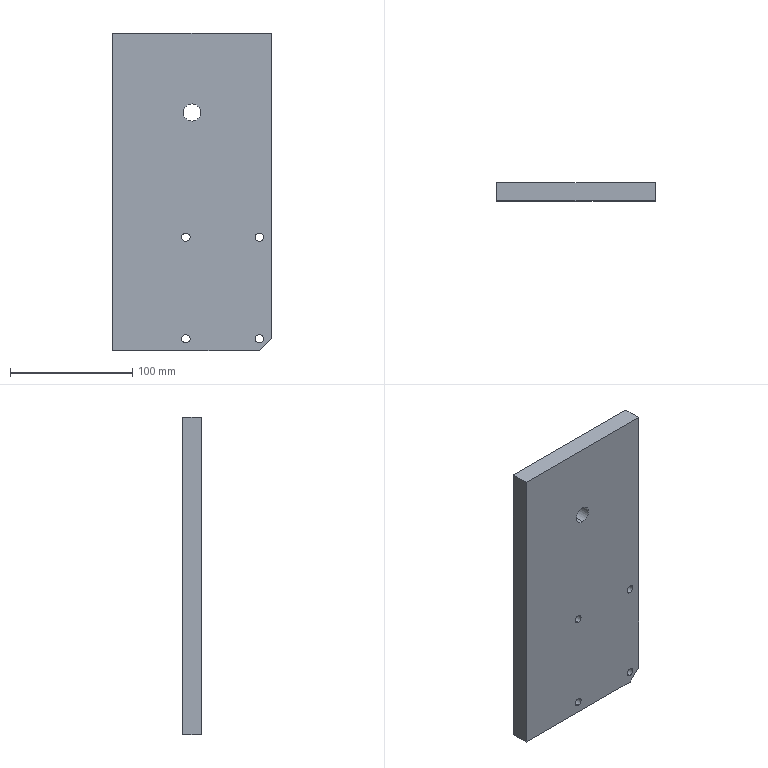Part | STEP file | PN_0001_default<by machining> | 1 solid | 17 faces | box 130 x 15 x 260 mm | volume 501762 mm3 | cylinder 10 | plane 7 | commonest cylinder face diameters 6.8 x8 14 x2
STEP:
#1=CARTESIAN_POINT('',(0.,0.,0.));
#2=DIRECTION('',(0.,0.,1.));
#3=DIRECTION('',(1.,0.,0.));
#4=AXIS2_PLACEMENT_3D('',#1,#2,#3);
#5=CARTESIAN_POINT('',(-180.,-25.,846.6));
#6=VERTEX_POINT('',#5);
#7=CARTESIAN_POINT('',(-180.,-40.,846.6));
#8=VERTEX_POINT('',#7);
#9=CARTESIAN_POINT('',(-180.,-40.,846.6));
#10=DIRECTION('',(0.,-1.,0.));
#11=VECTOR('',#10,1.);
#12=LINE('',#9,#11);
#13=CARTESIAN_POINT('',(-180.,-40.,850.));
#14=DIRECTION('',(0.,-1.,0.));
#15=DIRECTION('',(0.,0.,-1.));
#16=AXIS2_PLACEMENT_3D('',#13,#14,#15);
#17=CYLINDRICAL_SURFACE('',#16,3.4);
#18=CARTESIAN_POINT('',(6.283,0.));
#19=DIRECTION('',(0.,1.));
#20=VECTOR('',#19,1.);
#21=LINE('',#18,#20);
#22=(GEOMETRIC_REPRESENTATION_CONTEXT(2)PARAMETRIC_REPRESENTATION_CONTEXT()REPRESENTATION_CONTEXT('',''));
#23=DEFINITIONAL_REPRESENTATION('',(#21),#22);
#24=PCURVE('',#17,#23);
#25=CARTESIAN_POINT('',(-180.,-40.,850.));
#26=DIRECTION('',(0.,-1.,0.));
#27=DIRECTION('',(0.,0.,-1.));
#28=AXIS2_PLACEMENT_3D('',#25,#26,#27);
#29=CYLINDRICAL_SURFACE('',#28,3.4);
#30=CARTESIAN_POINT('',(0.,0.));
#31=DIRECTION('',(0.,1.));
#32=VECTOR('',#31,1.);
#33=LINE('',#30,#32);
#34=(GEOMETRIC_REPRESENTATION_CONTEXT(2)PARAMETRIC_REPRESENTATION_CONTEXT()REPRESENTATION_CONTEXT('',''));
#35=DEFINITIONAL_REPRESENTATION('',(#33),#34);
#36=PCURVE('',#29,#35);
#37=SURFACE_CURVE('',#12,(#24,#36),.PCURVE_S1.);
#38=EDGE_CURVE('',#6,#8,#37,.T.);
#39=ORIENTED_EDGE('',*,*,#38,.T.);
#40=CARTESIAN_POINT('',(-180.,-40.,853.4));
#41=VERTEX_POINT('',#40);
#42=CARTESIAN_POINT('',(-180.,-40.,850.));
#43=DIRECTION('',(0.,-1.,0.));
#44=DIRECTION('',(0.,0.,-1.));
#45=AXIS2_PLACEMENT_3D('',#42,#43,#44);
#46=CIRCLE('',#45,3.4);
#47=CARTESIAN_POINT('',(0.,0.));
#48=DIRECTION('',(1.,0.));
#49=VECTOR('',#48,1.);
#50=LINE('',#47,#49);
#51=(GEOMETRIC_REPRESENTATION_CONTEXT(2)PARAMETRIC_REPRESENTATION_CONTEXT()REPRESENTATION_CONTEXT('',''));
#52=DEFINITIONAL_REPRESENTATION('',(#50),#51);
#53=PCURVE('',#17,#52);
#54=CARTESIAN_POINT('',(0.,-40.,0.));
#55=DIRECTION('',(0.,-1.,0.));
#56=DIRECTION('',(0.,0.,-1.));
#57=AXIS2_PLACEMENT_3D('',#54,#55,#56);
#58=PLANE('',#57);
#59=CARTESIAN_POINT('',(-850.,-180.));
#60=DIRECTION('',(1.,0.));
#61=AXIS2_PLACEMENT_2D('',#59,#60);
#62=CIRCLE('',#61,3.4);
#63=(GEOMETRIC_REPRESENTATION_CONTEXT(2)PARAMETRIC_REPRESENTATION_CONTEXT()REPRESENTATION_CONTEXT('',''));
#64=DEFINITIONAL_REPRESENTATION('',(#62),#63);
#65=PCURVE('',#58,#64);
#66=SURFACE_CURVE('',#46,(#53,#65),.PCURVE_S1.);
#67=EDGE_CURVE('',#41,#8,#66,.T.);
#68=ORIENTED_EDGE('',*,*,#67,.F.);
#69=CARTESIAN_POINT('',(-180.,-25.,853.4));
#70=VERTEX_POINT('',#69);
#71=CARTESIAN_POINT('',(-180.,-40.,853.4));
#72=DIRECTION('',(0.,-1.,0.));
#73=VECTOR('',#72,1.);
#74=LINE('',#71,#73);
#75=CARTESIAN_POINT('',(3.142,0.));
#76=DIRECTION('',(0.,1.));
#77=VECTOR('',#76,1.);
#78=LINE('',#75,#77);
#79=(GEOMETRIC_REPRESENTATION_CONTEXT(2)PARAMETRIC_REPRESENTATION_CONTEXT()REPRESENTATION_CONTEXT('',''));
#80=DEFINITIONAL_REPRESENTATION('',(#78),#79);
#81=PCURVE('',#17,#80);
#82=CARTESIAN_POINT('',(3.142,0.));
#83=DIRECTION('',(0.,1.));
#84=VECTOR('',#83,1.);
#85=LINE('',#82,#84);
#86=(GEOMETRIC_REPRESENTATION_CONTEXT(2)PARAMETRIC_REPRESENTATION_CONTEXT()REPRESENTATION_CONTEXT('',''));
#87=DEFINITIONAL_REPRESENTATION('',(#85),#86);
#88=PCURVE('',#29,#87);
#89=SURFACE_CURVE('',#74,(#81,#88),.PCURVE_S1.);
#90=EDGE_CURVE('',#70,#41,#89,.T.);
#91=ORIENTED_EDGE('',*,*,#90,.F.);
#92=CARTESIAN_POINT('',(-180.,-25.,850.));
#93=DIRECTION('',(0.,-1.,0.));
#94=DIRECTION('',(0.,0.,-1.));
#95=AXIS2_PLACEMENT_3D('',#92,#93,#94);
#96=CIRCLE('',#95,3.4);
#97=CARTESIAN_POINT('',(0.,-15.));
#98=DIRECTION('',(1.,0.));
#99=VECTOR('',#98,1.);
#100=LINE('',#97,#99);
#101=(GEOMETRIC_REPRESENTATION_CONTEXT(2)PARAMETRIC_REPRESENTATION_CONTEXT()REPRESENTATION_CONTEXT('',''));
#102=DEFINITIONAL_REPRESENTATION('',(#100),#101);
#103=PCURVE('',#17,#102);
#104=CARTESIAN_POINT('',(0.,-25.,0.));
#105=DIRECTION('',(0.,-1.,0.));
#106=DIRECTION('',(0.,0.,-1.));
#107=AXIS2_PLACEMENT_3D('',#104,#105,#106);
#108=PLANE('',#107);
#109=CARTESIAN_POINT('',(-850.,-180.));
#110=DIRECTION('',(1.,0.));
#111=AXIS2_PLACEMENT_2D('',#109,#110);
#112=CIRCLE('',#111,3.4);
#113=(GEOMETRIC_REPRESENTATION_CONTEXT(2)PARAMETRIC_REPRESENTATION_CONTEXT()REPRESENTATION_CONTEXT('',''));
#114=DEFINITIONAL_REPRESENTATION('',(#112),#113);
#115=PCURVE('',#108,#114);
#116=SURFACE_CURVE('',#96,(#103,#115),.PCURVE_S1.);
#117=EDGE_CURVE('',#70,#6,#116,.T.);
#118=ORIENTED_EDGE('',*,*,#117,.T.);
#119=EDGE_LOOP('',(#39,#68,#91,#118));
#120=FACE_BOUND('',#119,.F.);
#121=ADVANCED_FACE('',(#120),#17,.F.);
#122=CARTESIAN_POINT('',(-180.,-25.,929.6));
#123=VERTEX_POINT('',#122);
#124=CARTESIAN_POINT('',(-180.,-40.,929.6));
#125=VERTEX_POINT('',#124);
#126=CARTESIAN_POINT('',(-180.,-40.,929.6));
#127=DIRECTION('',(0.,-1.,0.));
#128=VECTOR('',#127,1.);
#129=LINE('',#126,#128);
#130=CARTESIAN_POINT('',(-180.,-40.,933.));
#131=DIRECTION('',(0.,-1.,0.));
#132=DIRECTION('',(0.,0.,-1.));
#133=AXIS2_PLACEMENT_3D('',#130,#131,#132);
#134=CYLINDRICAL_SURFACE('',#133,3.4);
#135=CARTESIAN_POINT('',(6.283,0.));
#136=DIRECTION('',(0.,1.));
#137=VECTOR('',#136,1.);
#138=LINE('',#135,#137);
#139=(GEOMETRIC_REPRESENTATION_CONTEXT(2)PARAMETRIC_REPRESENTATION_CONTEXT()REPRESENTATION_CONTEXT('',''));
#140=DEFINITIONAL_REPRESENTATION('',(#138),#139);
#141=PCURVE('',#134,#140);
#142=CARTESIAN_POINT('',(-180.,-40.,933.));
#143=DIRECTION('',(0.,-1.,0.));
#144=DIRECTION('',(0.,0.,-1.));
#145=AXIS2_PLACEMENT_3D('',#142,#143,#144);
#146=CYLINDRICAL_SURFACE('',#145,3.4);
#147=CARTESIAN_POINT('',(0.,0.));
#148=DIRECTION('',(0.,1.));
#149=VECTOR('',#148,1.);
#150=LINE('',#147,#149);
#151=(GEOMETRIC_REPRESENTATION_CONTEXT(2)PARAMETRIC_REPRESENTATION_CONTEXT()REPRESENTATION_CONTEXT('',''));
#152=DEFINITIONAL_REPRESENTATION('',(#150),#151);
#153=PCURVE('',#146,#152);
#154=SURFACE_CURVE('',#129,(#141,#153),.PCURVE_S1.);
#155=EDGE_CURVE('',#123,#125,#154,.T.);
#156=ORIENTED_EDGE('',*,*,#155,.T.);
#157=CARTESIAN_POINT('',(-180.,-40.,936.4));
#158=VERTEX_POINT('',#157);
#159=CARTESIAN_POINT('',(-180.,-40.,933.));
#160=DIRECTION('',(0.,-1.,0.));
#161=DIRECTION('',(0.,0.,-1.));
#162=AXIS2_PLACEMENT_3D('',#159,#160,#161);
#163=CIRCLE('',#162,3.4);
#164=CARTESIAN_POINT('',(0.,0.));
#165=DIRECTION('',(1.,0.));
#166=VECTOR('',#165,1.);
#167=LINE('',#164,#166);
#168=(GEOMETRIC_REPRESENTATION_CONTEXT(2)PARAMETRIC_REPRESENTATION_CONTEXT()REPRESENTATION_CONTEXT('',''));
#169=DEFINITIONAL_REPRESENTATION('',(#167),#168);
#170=PCURVE('',#134,#169);
#171=CARTESIAN_POINT('',(-933.,-180.));
#172=DIRECTION('',(1.,0.));
#173=AXIS2_PLACEMENT_2D('',#171,#172);
#174=CIRCLE('',#173,3.4);
#175=(GEOMETRIC_REPRESENTATION_CONTEXT(2)PARAMETRIC_REPRESENTATION_CONTEXT()REPRESENTATION_CONTEXT('',''));
#176=DEFINITIONAL_REPRESENTATION('',(#174),#175);
#177=PCURVE('',#58,#176);
#178=SURFACE_CURVE('',#163,(#170,#177),.PCURVE_S1.);
#179=EDGE_CURVE('',#158,#125,#178,.T.);
#180=ORIENTED_EDGE('',*,*,#179,.F.);
#181=CARTESIAN_POINT('',(-180.,-25.,936.4));
#182=VERTEX_POINT('',#181);
#183=CARTESIAN_POINT('',(-180.,-40.,936.4));
#184=DIRECTION('',(0.,-1.,0.));
#185=VECTOR('',#184,1.);
#186=LINE('',#183,#185);
#187=CARTESIAN_POINT('',(3.142,0.));
#188=DIRECTION('',(0.,1.));
#189=VECTOR('',#188,1.);
#190=LINE('',#187,#189);
#191=(GEOMETRIC_REPRESENTATION_CONTEXT(2)PARAMETRIC_REPRESENTATION_CONTEXT()REPRESENTATION_CONTEXT('',''));
#192=DEFINITIONAL_REPRESENTATION('',(#190),#191);
#193=PCURVE('',#134,#192);
#194=CARTESIAN_POINT('',(3.142,0.));
#195=DIRECTION('',(0.,1.));
#196=VECTOR('',#195,1.);
#197=LINE('',#194,#196);
#198=(GEOMETRIC_REPRESENTATION_CONTEXT(2)PARAMETRIC_REPRESENTATION_CONTEXT()REPRESENTATION_CONTEXT('',''));
#199=DEFINITIONAL_REPRESENTATION('',(#197),#198);
#200=PCURVE('',#146,#199);
#201=SURFACE_CURVE('',#186,(#193,#200),.PCURVE_S1.);
#202=EDGE_CURVE('',#182,#158,#201,.T.);
#203=ORIENTED_EDGE('',*,*,#202,.F.);
#204=CARTESIAN_POINT('',(-180.,-25.,933.));
#205=DIRECTION('',(0.,-1.,0.));
#206=DIRECTION('',(0.,0.,-1.));
#207=AXIS2_PLACEMENT_3D('',#204,#205,#206);
#208=CIRCLE('',#207,3.4);
#209=CARTESIAN_POINT('',(0.,-15.));
#210=DIRECTION('',(1.,0.));
#211=VECTOR('',#210,1.);
#212=LINE('',#209,#211);
#213=(GEOMETRIC_REPRESENTATION_CONTEXT(2)PARAMETRIC_REPRESENTATION_CONTEXT()REPRESENTATION_CONTEXT('',''));
#214=DEFINITIONAL_REPRESENTATION('',(#212),#213);
#215=PCURVE('',#134,#214);
#216=CARTESIAN_POINT('',(-933.,-180.));
#217=DIRECTION('',(1.,0.));
#218=AXIS2_PLACEMENT_2D('',#216,#217);
#219=CIRCLE('',#218,3.4);
#220=(GEOMETRIC_REPRESENTATION_CONTEXT(2)PARAMETRIC_REPRESENTATION_CONTEXT()REPRESENTATION_CONTEXT('',''));
#221=DEFINITIONAL_REPRESENTATION('',(#219),#220);
#222=PCURVE('',#108,#221);
#223=SURFACE_CURVE('',#208,(#215,#222),.PCURVE_S1.);
#224=EDGE_CURVE('',#182,#123,#223,.T.);
#225=ORIENTED_EDGE('',*,*,#224,.T.);
#226=EDGE_LOOP('',(#156,#180,#203,#225));
#227=FACE_BOUND('',#226,.F.);
#228=ADVANCED_FACE('',(#227),#134,.F.);
#229=CARTESIAN_POINT('',(-240.,-25.,929.6));
#230=VERTEX_POINT('',#229);
#231=CARTESIAN_POINT('',(-240.,-40.,929.6));
#232=VERTEX_POINT('',#231);
#233=CARTESIAN_POINT('',(-240.,-40.,929.6));
#234=DIRECTION('',(0.,-1.,0.));
#235=VECTOR('',#234,1.);
#236=LINE('',#233,#235);
#237=CARTESIAN_POINT('',(-240.,-40.,933.));
#238=DIRECTION('',(0.,-1.,0.));
#239=DIRECTION('',(0.,0.,-1.));
#240=AXIS2_PLACEMENT_3D('',#237,#238,#239);
#241=CYLINDRICAL_SURFACE('',#240,3.4);
#242=CARTESIAN_POINT('',(6.283,0.));
#243=DIRECTION('',(0.,1.));
#244=VECTOR('',#243,1.);
#245=LINE('',#242,#244);
#246=(GEOMETRIC_REPRESENTATION_CONTEXT(2)PARAMETRIC_REPRESENTATION_CONTEXT()REPRESENTATION_CONTEXT('',''));
#247=DEFINITIONAL_REPRESENTATION('',(#245),#246);
#248=PCURVE('',#241,#247);
#249=CARTESIAN_POINT('',(-240.,-40.,933.));
#250=DIRECTION('',(0.,-1.,0.));
#251=DIRECTION('',(0.,0.,-1.));
#252=AXIS2_PLACEMENT_3D('',#249,#250,#251);
#253=CYLINDRICAL_SURFACE('',#252,3.4);
#254=CARTESIAN_POINT('',(0.,0.));
#255=DIRECTION('',(0.,1.));
#256=VECTOR('',#255,1.);
#257=LINE('',#254,#256);
#258=(GEOMETRIC_REPRESENTATION_CONTEXT(2)PARAMETRIC_REPRESENTATION_CONTEXT()REPRESENTATION_CONTEXT('',''));
#259=DEFINITIONAL_REPRESENTATION('',(#257),#258);
#260=PCURVE('',#253,#259);
#261=SURFACE_CURVE('',#236,(#248,#260),.PCURVE_S1.);
#262=EDGE_CURVE('',#230,#232,#261,.T.);
#263=ORIENTED_EDGE('',*,*,#262,.T.);
#264=CARTESIAN_POINT('',(-240.,-40.,936.4));
#265=VERTEX_POINT('',#264);
#266=CARTESIAN_POINT('',(-240.,-40.,933.));
#267=DIRECTION('',(0.,-1.,0.));
#268=DIRECTION('',(0.,0.,-1.));
#269=AXIS2_PLACEMENT_3D('',#266,#267,#268);
#270=CIRCLE('',#269,3.4);
#271=CARTESIAN_POINT('',(0.,0.));
#272=DIRECTION('',(1.,0.));
#273=VECTOR('',#272,1.);
#274=LINE('',#271,#273);
#275=(GEOMETRIC_REPRESENTATION_CONTEXT(2)PARAMETRIC_REPRESENTATION_CONTEXT()REPRESENTATION_CONTEXT('',''));
#276=DEFINITIONAL_REPRESENTATION('',(#274),#275);
#277=PCURVE('',#241,#276);
#278=CARTESIAN_POINT('',(-933.,-240.));
#279=DIRECTION('',(1.,0.));
#280=AXIS2_PLACEMENT_2D('',#278,#279);
#281=CIRCLE('',#280,3.4);
#282=(GEOMETRIC_REPRESENTATION_CONTEXT(2)PARAMETRIC_REPRESENTATION_CONTEXT()REPRESENTATION_CONTEXT('',''));
#283=DEFINITIONAL_REPRESENTATION('',(#281),#282);
#284=PCURVE('',#58,#283);
#285=SURFACE_CURVE('',#270,(#277,#284),.PCURVE_S1.);
#286=EDGE_CURVE('',#265,#232,#285,.T.);
#287=ORIENTED_EDGE('',*,*,#286,.F.);
#288=CARTESIAN_POINT('',(-240.,-25.,936.4));
#289=VERTEX_POINT('',#288);
#290=CARTESIAN_POINT('',(-240.,-40.,936.4));
#291=DIRECTION('',(0.,-1.,0.));
#292=VECTOR('',#291,1.);
#293=LINE('',#290,#292);
#294=CARTESIAN_POINT('',(3.142,0.));
#295=DIRECTION('',(0.,1.));
#296=VECTOR('',#295,1.);
#297=LINE('',#294,#296);
#298=(GEOMETRIC_REPRESENTATION_CONTEXT(2)PARAMETRIC_REPRESENTATION_CONTEXT()REPRESENTATION_CONTEXT('',''));
#299=DEFINITIONAL_REPRESENTATION('',(#297),#298);
#300=PCURVE('',#241,#299);
#301=CARTESIAN_POINT('',(3.142,0.));
#302=DIRECTION('',(0.,1.));
#303=VECTOR('',#302,1.);
#304=LINE('',#301,#303);
#305=(GEOMETRIC_REPRESENTATION_CONTEXT(2)PARAMETRIC_REPRESENTATION_CONTEXT()REPRESENTATION_CONTEXT('',''));
#306=DEFINITIONAL_REPRESENTATION('',(#304),#305);
#307=PCURVE('',#253,#306);
#308=SURFACE_CURVE('',#293,(#300,#307),.PCURVE_S1.);
#309=EDGE_CURVE('',#289,#265,#308,.T.);
#310=ORIENTED_EDGE('',*,*,#309,.F.);
#311=CARTESIAN_POINT('',(-240.,-25.,933.));
#312=DIRECTION('',(0.,-1.,0.));
#313=DIRECTION('',(0.,0.,-1.));
#314=AXIS2_PLACEMENT_3D('',#311,#312,#313);
#315=CIRCLE('',#314,3.4);
#316=CARTESIAN_POINT('',(0.,-15.));
#317=DIRECTION('',(1.,0.));
#318=VECTOR('',#317,1.);
#319=LINE('',#316,#318);
#320=(GEOMETRIC_REPRESENTATION_CONTEXT(2)PARAMETRIC_REPRESENTATION_CONTEXT()REPRESENTATION_CONTEXT('',''));
#321=DEFINITIONAL_REPRESENTATION('',(#319),#320);
#322=PCURVE('',#241,#321);
#323=CARTESIAN_POINT('',(-933.,-240.));
#324=DIRECTION('',(1.,0.));
#325=AXIS2_PLACEMENT_2D('',#323,#324);
#326=CIRCLE('',#325,3.4);
#327=(GEOMETRIC_REPRESENTATION_CONTEXT(2)PARAMETRIC_REPRESENTATION_CONTEXT()REPRESENTATION_CONTEXT('',''));
#328=DEFINITIONAL_REPRESENTATION('',(#326),#327);
#329=PCURVE('',#108,#328);
#330=SURFACE_CURVE('',#315,(#322,#329),.PCURVE_S1.);
#331=EDGE_CURVE('',#289,#230,#330,.T.);
#332=ORIENTED_EDGE('',*,*,#331,.T.);
#333=EDGE_LOOP('',(#263,#287,#310,#332));
#334=FACE_BOUND('',#333,.F.);
#335=ADVANCED_FACE('',(#334),#241,.F.);
#336=CARTESIAN_POINT('',(-240.,-25.,846.6));
#337=VERTEX_POINT('',#336);
#338=CARTESIAN_POINT('',(-240.,-40.,846.6));
#339=VERTEX_POINT('',#338);
#340=CARTESIAN_POINT('',(-240.,-40.,846.6));
#341=DIRECTION('',(0.,-1.,0.));
#342=VECTOR('',#341,1.);
#343=LINE('',#340,#342);
#344=CARTESIAN_POINT('',(-240.,-40.,850.));
#345=DIRECTION('',(0.,-1.,0.));
#346=DIRECTION('',(0.,0.,-1.));
#347=AXIS2_PLACEMENT_3D('',#344,#345,#346);
#348=CYLINDRICAL_SURFACE('',#347,3.4);
#349=CARTESIAN_POINT('',(6.283,0.));
#350=DIRECTION('',(0.,1.));
#351=VECTOR('',#350,1.);
#352=LINE('',#349,#351);
#353=(GEOMETRIC_REPRESENTATION_CONTEXT(2)PARAMETRIC_REPRESENTATION_CONTEXT()REPRESENTATION_CONTEXT('',''));
#354=DEFINITIONAL_REPRESENTATION('',(#352),#353);
#355=PCURVE('',#348,#354);
#356=CARTESIAN_POINT('',(-240.,-40.,850.));
#357=DIRECTION('',(0.,-1.,0.));
#358=DIRECTION('',(0.,0.,-1.));
#359=AXIS2_PLACEMENT_3D('',#356,#357,#358);
#360=CYLINDRICAL_SURFACE('',#359,3.4);
#361=CARTESIAN_POINT('',(0.,0.));
#362=DIRECTION('',(0.,1.));
#363=VECTOR('',#362,1.);
#364=LINE('',#361,#363);
#365=(GEOMETRIC_REPRESENTATION_CONTEXT(2)PARAMETRIC_REPRESENTATION_CONTEXT()REPRESENTATION_CONTEXT('',''));
#366=DEFINITIONAL_REPRESENTATION('',(#364),#365);
#367=PCURVE('',#360,#366);
#368=SURFACE_CURVE('',#343,(#355,#367),.PCURVE_S1.);
#369=EDGE_CURVE('',#337,#339,#368,.T.);
#370=ORIENTED_EDGE('',*,*,#369,.T.);
#371=CARTESIAN_POINT('',(-240.,-40.,853.4));
#372=VERTEX_POINT('',#371);
#373=CARTESIAN_POINT('',(-240.,-40.,850.));
#374=DIRECTION('',(0.,-1.,0.));
#375=DIRECTION('',(0.,0.,-1.));
#376=AXIS2_PLACEMENT_3D('',#373,#374,#375);
#377=CIRCLE('',#376,3.4);
#378=CARTESIAN_POINT('',(0.,0.));
#379=DIRECTION('',(1.,0.));
#380=VECTOR('',#379,1.);
#381=LINE('',#378,#380);
#382=(GEOMETRIC_REPRESENTATION_CONTEXT(2)PARAMETRIC_REPRESENTATION_CONTEXT()REPRESENTATION_CONTEXT('',''));
#383=DEFINITIONAL_REPRESENTATION('',(#381),#382);
#384=PCURVE('',#348,#383);
#385=CARTESIAN_POINT('',(-850.,-240.));
#386=DIRECTION('',(1.,0.));
#387=AXIS2_PLACEMENT_2D('',#385,#386);
#388=CIRCLE('',#387,3.4);
#389=(GEOMETRIC_REPRESENTATION_CONTEXT(2)PARAMETRIC_REPRESENTATION_CONTEXT()REPRESENTATION_CONTEXT('',''));
#390=DEFINITIONAL_REPRESENTATION('',(#388),#389);
#391=PCURVE('',#58,#390);
#392=SURFACE_CURVE('',#377,(#384,#391),.PCURVE_S1.);
#393=EDGE_CURVE('',#372,#339,#392,.T.);
#394=ORIENTED_EDGE('',*,*,#393,.F.);
#395=CARTESIAN_POINT('',(-240.,-25.,853.4));
#396=VERTEX_POINT('',#395);
#397=CARTESIAN_POINT('',(-240.,-40.,853.4));
#398=DIRECTION('',(0.,-1.,0.));
#399=VECTOR('',#398,1.);
#400=LINE('',#397,#399);
#401=CARTESIAN_POINT('',(3.142,0.));
#402=DIRECTION('',(0.,1.));
#403=VECTOR('',#402,1.);
#404=LINE('',#401,#403);
#405=(GEOMETRIC_REPRESENTATION_CONTEXT(2)PARAMETRIC_REPRESENTATION_CONTEXT()REPRESENTATION_CONTEXT('',''));
#406=DEFINITIONAL_REPRESENTATION('',(#404),#405);
#407=PCURVE('',#348,#406);
#408=CARTESIAN_POINT('',(3.142,0.));
#409=DIRECTION('',(0.,1.));
#410=VECTOR('',#409,1.);
#411=LINE('',#408,#410);
#412=(GEOMETRIC_REPRESENTATION_CONTEXT(2)PARAMETRIC_REPRESENTATION_CONTEXT()REPRESENTATION_CONTEXT('',''));
#413=DEFINITIONAL_REPRESENTATION('',(#411),#412);
#414=PCURVE('',#360,#413);
#415=SURFACE_CURVE('',#400,(#407,#414),.PCURVE_S1.);
#416=EDGE_CURVE('',#396,#372,#415,.T.);
#417=ORIENTED_EDGE('',*,*,#416,.F.);
#418=CARTESIAN_POINT('',(-240.,-25.,850.));
#419=DIRECTION('',(0.,-1.,0.));
#420=DIRECTION('',(0.,0.,-1.));
#421=AXIS2_PLACEMENT_3D('',#418,#419,#420);
#422=CIRCLE('',#421,3.4);
#423=CARTESIAN_POINT('',(0.,-15.));
#424=DIRECTION('',(1.,0.));
#425=VECTOR('',#424,1.);
#426=LINE('',#423,#425);
#427=(GEOMETRIC_REPRESENTATION_CONTEXT(2)PARAMETRIC_REPRESENTATION_CONTEXT()REPRESENTATION_CONTEXT('',''));
#428=DEFINITIONAL_REPRESENTATION('',(#426),#427);
#429=PCURVE('',#348,#428);
#430=CARTESIAN_POINT('',(-850.,-240.));
#431=DIRECTION('',(1.,0.));
#432=AXIS2_PLACEMENT_2D('',#430,#431);
#433=CIRCLE('',#432,3.4);
#434=(GEOMETRIC_REPRESENTATION_CONTEXT(2)PARAMETRIC_REPRESENTATION_CONTEXT()REPRESENTATION_CONTEXT('',''));
#435=DEFINITIONAL_REPRESENTATION('',(#433),#434);
#436=PCURVE('',#108,#435);
#437=SURFACE_CURVE('',#422,(#429,#436),.PCURVE_S1.);
#438=EDGE_CURVE('',#396,#337,#437,.T.);
#439=ORIENTED_EDGE('',*,*,#438,.T.);
#440=EDGE_LOOP('',(#370,#394,#417,#439));
#441=FACE_BOUND('',#440,.F.);
#442=ADVANCED_FACE('',(#441),#348,.F.);
#443=CARTESIAN_POINT('',(-235.,-25.,1028.));
#444=VERTEX_POINT('',#443);
#445=CARTESIAN_POINT('',(-235.,-40.,1028.));
#446=VERTEX_POINT('',#445);
#447=CARTESIAN_POINT('',(-235.,-40.,1028.));
#448=DIRECTION('',(0.,-1.,0.));
#449=VECTOR('',#448,1.);
#450=LINE('',#447,#449);
#451=CARTESIAN_POINT('',(-235.,-40.,1035.));
#452=DIRECTION('',(0.,-1.,0.));
#453=DIRECTION('',(0.,0.,-1.));
#454=AXIS2_PLACEMENT_3D('',#451,#452,#453);
#455=CYLINDRICAL_SURFACE('',#454,7.);
#456=CARTESIAN_POINT('',(6.283,0.));
#457=DIRECTION('',(0.,1.));
#458=VECTOR('',#457,1.);
#459=LINE('',#456,#458);
#460=(GEOMETRIC_REPRESENTATION_CONTEXT(2)PARAMETRIC_REPRESENTATION_CONTEXT()REPRESENTATION_CONTEXT('',''));
#461=DEFINITIONAL_REPRESENTATION('',(#459),#460);
#462=PCURVE('',#455,#461);
#463=CARTESIAN_POINT('',(-235.,-40.,1035.));
#464=DIRECTION('',(0.,-1.,0.));
#465=DIRECTION('',(0.,0.,-1.));
#466=AXIS2_PLACEMENT_3D('',#463,#464,#465);
#467=CYLINDRICAL_SURFACE('',#466,7.);
#468=CARTESIAN_POINT('',(0.,0.));
#469=DIRECTION('',(0.,1.));
#470=VECTOR('',#469,1.);
#471=LINE('',#468,#470);
#472=(GEOMETRIC_REPRESENTATION_CONTEXT(2)PARAMETRIC_REPRESENTATION_CONTEXT()REPRESENTATION_CONTEXT('',''));
#473=DEFINITIONAL_REPRESENTATION('',(#471),#472);
#474=PCURVE('',#467,#473);
#475=SURFACE_CURVE('',#450,(#462,#474),.PCURVE_S1.);
#476=EDGE_CURVE('',#444,#446,#475,.T.);
#477=ORIENTED_EDGE('',*,*,#476,.T.);
#478=CARTESIAN_POINT('',(-235.,-40.,1042.));
#479=VERTEX_POINT('',#478);
#480=CARTESIAN_POINT('',(-235.,-40.,1035.));
#481=DIRECTION('',(0.,-1.,0.));
#482=DIRECTION('',(0.,0.,-1.));
#483=AXIS2_PLACEMENT_3D('',#480,#481,#482);
#484=CIRCLE('',#483,7.);
#485=CARTESIAN_POINT('',(0.,0.));
#486=DIRECTION('',(1.,0.));
#487=VECTOR('',#486,1.);
#488=LINE('',#485,#487);
#489=(GEOMETRIC_REPRESENTATION_CONTEXT(2)PARAMETRIC_REPRESENTATION_CONTEXT()REPRESENTATION_CONTEXT('',''));
#490=DEFINITIONAL_REPRESENTATION('',(#488),#489);
#491=PCURVE('',#455,#490);
#492=CARTESIAN_POINT('',(-1035.,-235.));
#493=DIRECTION('',(1.,0.));
#494=AXIS2_PLACEMENT_2D('',#492,#493);
#495=CIRCLE('',#494,7.);
#496=(GEOMETRIC_REPRESENTATION_CONTEXT(2)PARAMETRIC_REPRESENTATION_CONTEXT()REPRESENTATION_CONTEXT('',''));
#497=DEFINITIONAL_REPRESENTATION('',(#495),#496);
#498=PCURVE('',#58,#497);
#499=SURFACE_CURVE('',#484,(#491,#498),.PCURVE_S1.);
#500=EDGE_CURVE('',#479,#446,#499,.T.);
#501=ORIENTED_EDGE('',*,*,#500,.F.);
#502=CARTESIAN_POINT('',(-235.,-25.,1042.));
#503=VERTEX_POINT('',#502);
#504=CARTESIAN_POINT('',(-235.,-40.,1042.));
#505=DIRECTION('',(0.,-1.,0.));
#506=VECTOR('',#505,1.);
#507=LINE('',#504,#506);
#508=CARTESIAN_POINT('',(3.142,0.));
#509=DIRECTION('',(0.,1.));
#510=VECTOR('',#509,1.);
#511=LINE('',#508,#510);
#512=(GEOMETRIC_REPRESENTATION_CONTEXT(2)PARAMETRIC_REPRESENTATION_CONTEXT()REPRESENTATION_CONTEXT('',''));
#513=DEFINITIONAL_REPRESENTATION('',(#511),#512);
#514=PCURVE('',#455,#513);
#515=CARTESIAN_POINT('',(3.142,0.));
#516=DIRECTION('',(0.,1.));
#517=VECTOR('',#516,1.);
#518=LINE('',#515,#517);
#519=(GEOMETRIC_REPRESENTATION_CONTEXT(2)PARAMETRIC_REPRESENTATION_CONTEXT()REPRESENTATION_CONTEXT('',''));
#520=DEFINITIONAL_REPRESENTATION('',(#518),#519);
#521=PCURVE('',#467,#520);
#522=SURFACE_CURVE('',#507,(#514,#521),.PCURVE_S1.);
#523=EDGE_CURVE('',#503,#479,#522,.T.);
#524=ORIENTED_EDGE('',*,*,#523,.F.);
#525=CARTESIAN_POINT('',(-235.,-25.,1035.));
#526=DIRECTION('',(0.,-1.,0.));
#527=DIRECTION('',(0.,0.,-1.));
#528=AXIS2_PLACEMENT_3D('',#525,#526,#527);
#529=CIRCLE('',#528,7.);
#530=CARTESIAN_POINT('',(0.,-15.));
#531=DIRECTION('',(1.,0.));
#532=VECTOR('',#531,1.);
#533=LINE('',#530,#532);
#534=(GEOMETRIC_REPRESENTATION_CONTEXT(2)PARAMETRIC_REPRESENTATION_CONTEXT()REPRESENTATION_CONTEXT('',''));
#535=DEFINITIONAL_REPRESENTATION('',(#533),#534);
#536=PCURVE('',#455,#535);
#537=CARTESIAN_POINT('',(-1035.,-235.));
#538=DIRECTION('',(1.,0.));
#539=AXIS2_PLACEMENT_2D('',#537,#538);
#540=CIRCLE('',#539,7.);
#541=(GEOMETRIC_REPRESENTATION_CONTEXT(2)PARAMETRIC_REPRESENTATION_CONTEXT()REPRESENTATION_CONTEXT('',''));
#542=DEFINITIONAL_REPRESENTATION('',(#540),#541);
#543=PCURVE('',#108,#542);
#544=SURFACE_CURVE('',#529,(#536,#543),.PCURVE_S1.);
#545=EDGE_CURVE('',#503,#444,#544,.T.);
#546=ORIENTED_EDGE('',*,*,#545,.T.);
#547=EDGE_LOOP('',(#477,#501,#524,#546));
#548=FACE_BOUND('',#547,.F.);
#549=ADVANCED_FACE('',(#548),#455,.F.);
#550=CARTESIAN_POINT('',(-300.,-25.,1100.));
#551=VERTEX_POINT('',#550);
#552=CARTESIAN_POINT('',(-300.,-25.,840.));
#553=VERTEX_POINT('',#552);
#554=CARTESIAN_POINT('',(-300.,-25.,1100.));
#555=DIRECTION('',(0.,0.,-1.));
#556=VECTOR('',#555,1.);
#557=LINE('',#554,#556);
#558=CARTESIAN_POINT('',(-300.,-40.,1100.));
#559=DIRECTION('',(1.,0.,0.));
#560=DIRECTION('',(0.,1.,0.));
#561=AXIS2_PLACEMENT_3D('',#558,#559,#560);
#562=PLANE('',#561);
#563=CARTESIAN_POINT('',(15.,0.));
#564=DIRECTION('',(0.,-1.));
#565=VECTOR('',#564,1.);
#566=LINE('',#563,#565);
#567=(GEOMETRIC_REPRESENTATION_CONTEXT(2)PARAMETRIC_REPRESENTATION_CONTEXT()REPRESENTATION_CONTEXT('',''));
#568=DEFINITIONAL_REPRESENTATION('',(#566),#567);
#569=PCURVE('',#562,#568);
#570=CARTESIAN_POINT('',(-1100.,-300.));
#571=DIRECTION('',(1.,0.));
#572=VECTOR('',#571,1.);
#573=LINE('',#570,#572);
#574=(GEOMETRIC_REPRESENTATION_CONTEXT(2)PARAMETRIC_REPRESENTATION_CONTEXT()REPRESENTATION_CONTEXT('',''));
#575=DEFINITIONAL_REPRESENTATION('',(#573),#574);
#576=PCURVE('',#108,#575);
#577=SURFACE_CURVE('',#557,(#569,#576),.PCURVE_S1.);
#578=EDGE_CURVE('',#551,#553,#577,.T.);
#579=ORIENTED_EDGE('',*,*,#578,.T.);
#580=CARTESIAN_POINT('',(-300.,-40.,840.));
#581=VERTEX_POINT('',#580);
#582=CARTESIAN_POINT('',(-300.,-40.,840.));
#583=DIRECTION('',(0.,1.,0.));
#584=VECTOR('',#583,1.);
#585=LINE('',#582,#584);
#586=CARTESIAN_POINT('',(0.,-260.));
#587=DIRECTION('',(1.,0.));
#588=VECTOR('',#587,1.);
#589=LINE('',#586,#588);
#590=(GEOMETRIC_REPRESENTATION_CONTEXT(2)PARAMETRIC_REPRESENTATION_CONTEXT()REPRESENTATION_CONTEXT('',''));
#591=DEFINITIONAL_REPRESENTATION('',(#589),#590);
#592=PCURVE('',#562,#591);
#593=CARTESIAN_POINT('',(-300.,-40.,840.));
#594=DIRECTION('',(0.,0.,1.));
#595=DIRECTION('',(0.,-1.,0.));
#596=AXIS2_PLACEMENT_3D('',#593,#594,#595);
#597=PLANE('',#596);
#598=CARTESIAN_POINT('',(0.,0.));
#599=DIRECTION('',(-1.,0.));
#600=VECTOR('',#599,1.);
#601=LINE('',#598,#600);
#602=(GEOMETRIC_REPRESENTATION_CONTEXT(2)PARAMETRIC_REPRESENTATION_CONTEXT()REPRESENTATION_CONTEXT('',''));
#603=DEFINITIONAL_REPRESENTATION('',(#601),#602);
#604=PCURVE('',#597,#603);
#605=SURFACE_CURVE('',#585,(#592,#604),.PCURVE_S1.);
#606=EDGE_CURVE('',#581,#553,#605,.T.);
#607=ORIENTED_EDGE('',*,*,#606,.F.);
#608=CARTESIAN_POINT('',(-300.,-40.,1100.));
#609=VERTEX_POINT('',#608);
#610=CARTESIAN_POINT('',(-300.,-40.,1100.));
#611=DIRECTION('',(0.,0.,-1.));
#612=VECTOR('',#611,1.);
#613=LINE('',#610,#612);
#614=CARTESIAN_POINT('',(0.,0.));
#615=DIRECTION('',(0.,-1.));
#616=VECTOR('',#615,1.);
#617=LINE('',#614,#616);
#618=(GEOMETRIC_REPRESENTATION_CONTEXT(2)PARAMETRIC_REPRESENTATION_CONTEXT()REPRESENTATION_CONTEXT('',''));
#619=DEFINITIONAL_REPRESENTATION('',(#617),#618);
#620=PCURVE('',#562,#619);
#621=CARTESIAN_POINT('',(-1100.,-300.));
#622=DIRECTION('',(1.,0.));
#623=VECTOR('',#622,1.);
#624=LINE('',#621,#623);
#625=(GEOMETRIC_REPRESENTATION_CONTEXT(2)PARAMETRIC_REPRESENTATION_CONTEXT()REPRESENTATION_CONTEXT('',''));
#626=DEFINITIONAL_REPRESENTATION('',(#624),#625);
#627=PCURVE('',#58,#626);
#628=SURFACE_CURVE('',#613,(#620,#627),.PCURVE_S1.);
#629=EDGE_CURVE('',#609,#581,#628,.T.);
#630=ORIENTED_EDGE('',*,*,#629,.F.);
#631=CARTESIAN_POINT('',(-300.,-40.,1100.));
#632=DIRECTION('',(0.,1.,0.));
#633=VECTOR('',#632,1.);
#634=LINE('',#631,#633);
#635=CARTESIAN_POINT('',(0.,0.));
#636=DIRECTION('',(1.,0.));
#637=VECTOR('',#636,1.);
#638=LINE('',#635,#637);
#639=(GEOMETRIC_REPRESENTATION_CONTEXT(2)PARAMETRIC_REPRESENTATION_CONTEXT()REPRESENTATION_CONTEXT('',''));
#640=DEFINITIONAL_REPRESENTATION('',(#638),#639);
#641=PCURVE('',#562,#640);
#642=CARTESIAN_POINT('',(-300.,-40.,1100.));
#643=DIRECTION('',(0.,0.,-1.));
#644=DIRECTION('',(0.,1.,0.));
#645=AXIS2_PLACEMENT_3D('',#642,#643,#644);
#646=PLANE('',#645);
#647=CARTESIAN_POINT('',(0.,0.));
#648=DIRECTION('',(1.,0.));
#649=VECTOR('',#648,1.);
#650=LINE('',#647,#649);
#651=(GEOMETRIC_REPRESENTATION_CONTEXT(2)PARAMETRIC_REPRESENTATION_CONTEXT()REPRESENTATION_CONTEXT('',''));
#652=DEFINITIONAL_REPRESENTATION('',(#650),#651);
#653=PCURVE('',#646,#652);
#654=SURFACE_CURVE('',#634,(#641,#653),.PCURVE_S1.);
#655=EDGE_CURVE('',#609,#551,#654,.T.);
#656=ORIENTED_EDGE('',*,*,#655,.T.);
#657=EDGE_LOOP('',(#579,#607,#630,#656));
#658=FACE_BOUND('',#657,.T.);
#659=ADVANCED_FACE('',(#658),#562,.F.);
#660=CARTESIAN_POINT('',(-180.,-25.,840.));
#661=VERTEX_POINT('',#660);
#662=CARTESIAN_POINT('',(-300.,-25.,840.));
#663=DIRECTION('',(1.,0.,0.));
#664=VECTOR('',#663,1.);
#665=LINE('',#662,#664);
#666=CARTESIAN_POINT('',(-15.,0.));
#667=DIRECTION('',(0.,1.));
#668=VECTOR('',#667,1.);
#669=LINE('',#666,#668);
#670=(GEOMETRIC_REPRESENTATION_CONTEXT(2)PARAMETRIC_REPRESENTATION_CONTEXT()REPRESENTATION_CONTEXT('',''));
#671=DEFINITIONAL_REPRESENTATION('',(#669),#670);
#672=PCURVE('',#597,#671);
#673=CARTESIAN_POINT('',(-840.,-300.));
#674=DIRECTION('',(0.,1.));
#675=VECTOR('',#674,1.);
#676=LINE('',#673,#675);
#677=(GEOMETRIC_REPRESENTATION_CONTEXT(2)PARAMETRIC_REPRESENTATION_CONTEXT()REPRESENTATION_CONTEXT('',''));
#678=DEFINITIONAL_REPRESENTATION('',(#676),#677);
#679=PCURVE('',#108,#678);
#680=SURFACE_CURVE('',#665,(#672,#679),.PCURVE_S1.);
#681=EDGE_CURVE('',#553,#661,#680,.T.);
#682=ORIENTED_EDGE('',*,*,#681,.T.);
#683=CARTESIAN_POINT('',(-180.,-40.,840.));
#684=VERTEX_POINT('',#683);
#685=CARTESIAN_POINT('',(-180.,-40.,840.));
#686=DIRECTION('',(0.,1.,0.));
#687=VECTOR('',#686,1.);
#688=LINE('',#685,#687);
#689=CARTESIAN_POINT('',(0.,120.));
#690=DIRECTION('',(-1.,0.));
#691=VECTOR('',#690,1.);
#692=LINE('',#689,#691);
#693=(GEOMETRIC_REPRESENTATION_CONTEXT(2)PARAMETRIC_REPRESENTATION_CONTEXT()REPRESENTATION_CONTEXT('',''));
#694=DEFINITIONAL_REPRESENTATION('',(#692),#693);
#695=PCURVE('',#597,#694);
#696=CARTESIAN_POINT('',(-180.,-40.,840.));
#697=DIRECTION('',(-0.7071,0.,0.7071));
#698=DIRECTION('',(0.7071,0.,0.7071));
#699=AXIS2_PLACEMENT_3D('',#696,#697,#698);
#700=PLANE('',#699);
#701=CARTESIAN_POINT('',(0.,0.));
#702=DIRECTION('',(0.,1.));
#703=VECTOR('',#702,1.);
#704=LINE('',#701,#703);
#705=(GEOMETRIC_REPRESENTATION_CONTEXT(2)PARAMETRIC_REPRESENTATION_CONTEXT()REPRESENTATION_CONTEXT('',''));
#706=DEFINITIONAL_REPRESENTATION('',(#704),#705);
#707=PCURVE('',#700,#706);
#708=SURFACE_CURVE('',#688,(#695,#707),.PCURVE_S1.);
#709=EDGE_CURVE('',#684,#661,#708,.T.);
#710=ORIENTED_EDGE('',*,*,#709,.F.);
#711=CARTESIAN_POINT('',(-300.,-40.,840.));
#712=DIRECTION('',(1.,0.,0.));
#713=VECTOR('',#712,1.);
#714=LINE('',#711,#713);
#715=CARTESIAN_POINT('',(0.,0.));
#716=DIRECTION('',(0.,1.));
#717=VECTOR('',#716,1.);
#718=LINE('',#715,#717);
#719=(GEOMETRIC_REPRESENTATION_CONTEXT(2)PARAMETRIC_REPRESENTATION_CONTEXT()REPRESENTATION_CONTEXT('',''));
#720=DEFINITIONAL_REPRESENTATION('',(#718),#719);
#721=PCURVE('',#597,#720);
#722=CARTESIAN_POINT('',(-840.,-300.));
#723=DIRECTION('',(0.,1.));
#724=VECTOR('',#723,1.);
#725=LINE('',#722,#724);
#726=(GEOMETRIC_REPRESENTATION_CONTEXT(2)PARAMETRIC_REPRESENTATION_CONTEXT()REPRESENTATION_CONTEXT('',''));
#727=DEFINITIONAL_REPRESENTATION('',(#725),#726);
#728=PCURVE('',#58,#727);
#729=SURFACE_CURVE('',#714,(#721,#728),.PCURVE_S1.);
#730=EDGE_CURVE('',#581,#684,#729,.T.);
#731=ORIENTED_EDGE('',*,*,#730,.F.);
#732=ORIENTED_EDGE('',*,*,#606,.T.);
#733=EDGE_LOOP('',(#682,#710,#731,#732));
#734=FACE_BOUND('',#733,.T.);
#735=ADVANCED_FACE('',(#734),#597,.F.);
#736=CARTESIAN_POINT('',(-170.,-25.,850.));
#737=VERTEX_POINT('',#736);
#738=CARTESIAN_POINT('',(-180.,-25.,840.));
#739=DIRECTION('',(0.7071,0.,0.7071));
#740=VECTOR('',#739,1.);
#741=LINE('',#738,#740);
#742=CARTESIAN_POINT('',(0.,15.));
#743=DIRECTION('',(1.,0.));
#744=VECTOR('',#743,1.);
#745=LINE('',#742,#744);
#746=(GEOMETRIC_REPRESENTATION_CONTEXT(2)PARAMETRIC_REPRESENTATION_CONTEXT()REPRESENTATION_CONTEXT('',''));
#747=DEFINITIONAL_REPRESENTATION('',(#745),#746);
#748=PCURVE('',#700,#747);
#749=CARTESIAN_POINT('',(-840.,-180.));
#750=DIRECTION('',(-0.7071,0.7071));
#751=VECTOR('',#750,1.);
#752=LINE('',#749,#751);
#753=(GEOMETRIC_REPRESENTATION_CONTEXT(2)PARAMETRIC_REPRESENTATION_CONTEXT()REPRESENTATION_CONTEXT('',''));
#754=DEFINITIONAL_REPRESENTATION('',(#752),#753);
#755=PCURVE('',#108,#754);
#756=SURFACE_CURVE('',#741,(#748,#755),.PCURVE_S1.);
#757=EDGE_CURVE('',#661,#737,#756,.T.);
#758=ORIENTED_EDGE('',*,*,#757,.T.);
#759=CARTESIAN_POINT('',(-170.,-40.,850.));
#760=VERTEX_POINT('',#759);
#761=CARTESIAN_POINT('',(-170.,-40.,850.));
#762=DIRECTION('',(0.,1.,0.));
#763=VECTOR('',#762,1.);
#764=LINE('',#761,#763);
#765=CARTESIAN_POINT('',(14.142,0.));
#766=DIRECTION('',(0.,1.));
#767=VECTOR('',#766,1.);
#768=LINE('',#765,#767);
#769=(GEOMETRIC_REPRESENTATION_CONTEXT(2)PARAMETRIC_REPRESENTATION_CONTEXT()REPRESENTATION_CONTEXT('',''));
#770=DEFINITIONAL_REPRESENTATION('',(#768),#769);
#771=PCURVE('',#700,#770);
#772=CARTESIAN_POINT('',(-170.,-40.,1100.));
#773=DIRECTION('',(-1.,0.,0.));
#774=DIRECTION('',(0.,-1.,0.));
#775=AXIS2_PLACEMENT_3D('',#772,#773,#774);
#776=PLANE('',#775);
#777=CARTESIAN_POINT('',(0.,-250.));
#778=DIRECTION('',(-1.,0.));
#779=VECTOR('',#778,1.);
#780=LINE('',#777,#779);
#781=(GEOMETRIC_REPRESENTATION_CONTEXT(2)PARAMETRIC_REPRESENTATION_CONTEXT()REPRESENTATION_CONTEXT('',''));
#782=DEFINITIONAL_REPRESENTATION('',(#780),#781);
#783=PCURVE('',#776,#782);
#784=SURFACE_CURVE('',#764,(#771,#783),.PCURVE_S1.);
#785=EDGE_CURVE('',#760,#737,#784,.T.);
#786=ORIENTED_EDGE('',*,*,#785,.F.);
#787=CARTESIAN_POINT('',(-180.,-40.,840.));
#788=DIRECTION('',(0.7071,0.,0.7071));
#789=VECTOR('',#788,1.);
#790=LINE('',#787,#789);
#791=CARTESIAN_POINT('',(0.,0.));
#792=DIRECTION('',(1.,0.));
#793=VECTOR('',#792,1.);
#794=LINE('',#791,#793);
#795=(GEOMETRIC_REPRESENTATION_CONTEXT(2)PARAMETRIC_REPRESENTATION_CONTEXT()REPRESENTATION_CONTEXT('',''));
#796=DEFINITIONAL_REPRESENTATION('',(#794),#795);
#797=PCURVE('',#700,#796);
#798=CARTESIAN_POINT('',(-840.,-180.));
#799=DIRECTION('',(-0.7071,0.7071));
#800=VECTOR('',#799,1.);
#801=LINE('',#798,#800);
#802=(GEOMETRIC_REPRESENTATION_CONTEXT(2)PARAMETRIC_REPRESENTATION_CONTEXT()REPRESENTATION_CONTEXT('',''));
#803=DEFINITIONAL_REPRESENTATION('',(#801),#802);
#804=PCURVE('',#58,#803);
#805=SURFACE_CURVE('',#790,(#797,#804),.PCURVE_S1.);
#806=EDGE_CURVE('',#684,#760,#805,.T.);
#807=ORIENTED_EDGE('',*,*,#806,.F.);
#808=ORIENTED_EDGE('',*,*,#709,.T.);
#809=EDGE_LOOP('',(#758,#786,#807,#808));
#810=FACE_BOUND('',#809,.T.);
#811=ADVANCED_FACE('',(#810),#700,.F.);
#812=CARTESIAN_POINT('',(-170.,-25.,1100.));
#813=VERTEX_POINT('',#812);
#814=CARTESIAN_POINT('',(-170.,-25.,1100.));
#815=DIRECTION('',(0.,0.,1.));
#816=VECTOR('',#815,1.);
#817=LINE('',#814,#816);
#818=CARTESIAN_POINT('',(-15.,0.));
#819=DIRECTION('',(0.,1.));
#820=VECTOR('',#819,1.);
#821=LINE('',#818,#820);
#822=(GEOMETRIC_REPRESENTATION_CONTEXT(2)PARAMETRIC_REPRESENTATION_CONTEXT()REPRESENTATION_CONTEXT('',''));
#823=DEFINITIONAL_REPRESENTATION('',(#821),#822);
#824=PCURVE('',#776,#823);
#825=CARTESIAN_POINT('',(-1100.,-170.));
#826=DIRECTION('',(-1.,0.));
#827=VECTOR('',#826,1.);
#828=LINE('',#825,#827);
#829=(GEOMETRIC_REPRESENTATION_CONTEXT(2)PARAMETRIC_REPRESENTATION_CONTEXT()REPRESENTATION_CONTEXT('',''));
#830=DEFINITIONAL_REPRESENTATION('',(#828),#829);
#831=PCURVE('',#108,#830);
#832=SURFACE_CURVE('',#817,(#824,#831),.PCURVE_S1.);
#833=EDGE_CURVE('',#737,#813,#832,.T.);
#834=ORIENTED_EDGE('',*,*,#833,.T.);
#835=CARTESIAN_POINT('',(-170.,-40.,1100.));
#836=VERTEX_POINT('',#835);
#837=CARTESIAN_POINT('',(-170.,-40.,1100.));
#838=DIRECTION('',(0.,1.,0.));
#839=VECTOR('',#838,1.);
#840=LINE('',#837,#839);
#841=CARTESIAN_POINT('',(0.,0.));
#842=DIRECTION('',(-1.,0.));
#843=VECTOR('',#842,1.);
#844=LINE('',#841,#843);
#845=(GEOMETRIC_REPRESENTATION_CONTEXT(2)PARAMETRIC_REPRESENTATION_CONTEXT()REPRESENTATION_CONTEXT('',''));
#846=DEFINITIONAL_REPRESENTATION('',(#844),#845);
#847=PCURVE('',#776,#846);
#848=CARTESIAN_POINT('',(0.,130.));
#849=DIRECTION('',(1.,0.));
#850=VECTOR('',#849,1.);
#851=LINE('',#848,#850);
#852=(GEOMETRIC_REPRESENTATION_CONTEXT(2)PARAMETRIC_REPRESENTATION_CONTEXT()REPRESENTATION_CONTEXT('',''));
#853=DEFINITIONAL_REPRESENTATION('',(#851),#852);
#854=PCURVE('',#646,#853);
#855=SURFACE_CURVE('',#840,(#847,#854),.PCURVE_S1.);
#856=EDGE_CURVE('',#836,#813,#855,.T.);
#857=ORIENTED_EDGE('',*,*,#856,.F.);
#858=CARTESIAN_POINT('',(-170.,-40.,1100.));
#859=DIRECTION('',(0.,0.,1.));
#860=VECTOR('',#859,1.);
#861=LINE('',#858,#860);
#862=CARTESIAN_POINT('',(0.,0.));
#863=DIRECTION('',(0.,1.));
#864=VECTOR('',#863,1.);
#865=LINE('',#862,#864);
#866=(GEOMETRIC_REPRESENTATION_CONTEXT(2)PARAMETRIC_REPRESENTATION_CONTEXT()REPRESENTATION_CONTEXT('',''));
#867=DEFINITIONAL_REPRESENTATION('',(#865),#866);
#868=PCURVE('',#776,#867);
#869=CARTESIAN_POINT('',(-1100.,-170.));
#870=DIRECTION('',(-1.,0.));
#871=VECTOR('',#870,1.);
#872=LINE('',#869,#871);
#873=(GEOMETRIC_REPRESENTATION_CONTEXT(2)PARAMETRIC_REPRESENTATION_CONTEXT()REPRESENTATION_CONTEXT('',''));
#874=DEFINITIONAL_REPRESENTATION('',(#872),#873);
#875=PCURVE('',#58,#874);
#876=SURFACE_CURVE('',#861,(#868,#875),.PCURVE_S1.);
#877=EDGE_CURVE('',#760,#836,#876,.T.);
#878=ORIENTED_EDGE('',*,*,#877,.F.);
#879=ORIENTED_EDGE('',*,*,#785,.T.);
#880=EDGE_LOOP('',(#834,#857,#878,#879));
#881=FACE_BOUND('',#880,.T.);
#882=ADVANCED_FACE('',(#881),#776,.F.);
#883=CARTESIAN_POINT('',(-300.,-25.,1100.));
#884=DIRECTION('',(-1.,0.,0.));
#885=VECTOR('',#884,1.);
#886=LINE('',#883,#885);
#887=CARTESIAN_POINT('',(15.,0.));
#888=DIRECTION('',(0.,-1.));
#889=VECTOR('',#888,1.);
#890=LINE('',#887,#889);
#891=(GEOMETRIC_REPRESENTATION_CONTEXT(2)PARAMETRIC_REPRESENTATION_CONTEXT()REPRESENTATION_CONTEXT('',''));
#892=DEFINITIONAL_REPRESENTATION('',(#890),#891);
#893=PCURVE('',#646,#892);
#894=CARTESIAN_POINT('',(-1100.,-300.));
#895=DIRECTION('',(0.,-1.));
#896=VECTOR('',#895,1.);
#897=LINE('',#894,#896);
#898=(GEOMETRIC_REPRESENTATION_CONTEXT(2)PARAMETRIC_REPRESENTATION_CONTEXT()REPRESENTATION_CONTEXT('',''));
#899=DEFINITIONAL_REPRESENTATION('',(#897),#898);
#900=PCURVE('',#108,#899);
#901=SURFACE_CURVE('',#886,(#893,#900),.PCURVE_S1.);
#902=EDGE_CURVE('',#813,#551,#901,.T.);
#903=ORIENTED_EDGE('',*,*,#902,.T.);
#904=ORIENTED_EDGE('',*,*,#655,.F.);
#905=CARTESIAN_POINT('',(-300.,-40.,1100.));
#906=DIRECTION('',(-1.,0.,0.));
#907=VECTOR('',#906,1.);
#908=LINE('',#905,#907);
#909=CARTESIAN_POINT('',(0.,0.));
#910=DIRECTION('',(0.,-1.));
#911=VECTOR('',#910,1.);
#912=LINE('',#909,#911);
#913=(GEOMETRIC_REPRESENTATION_CONTEXT(2)PARAMETRIC_REPRESENTATION_CONTEXT()REPRESENTATION_CONTEXT('',''));
#914=DEFINITIONAL_REPRESENTATION('',(#912),#913);
#915=PCURVE('',#646,#914);
#916=CARTESIAN_POINT('',(-1100.,-300.));
#917=DIRECTION('',(0.,-1.));
#918=VECTOR('',#917,1.);
#919=LINE('',#916,#918);
#920=(GEOMETRIC_REPRESENTATION_CONTEXT(2)PARAMETRIC_REPRESENTATION_CONTEXT()REPRESENTATION_CONTEXT('',''));
#921=DEFINITIONAL_REPRESENTATION('',(#919),#920);
#922=PCURVE('',#58,#921);
#923=SURFACE_CURVE('',#908,(#915,#922),.PCURVE_S1.);
#924=EDGE_CURVE('',#836,#609,#923,.T.);
#925=ORIENTED_EDGE('',*,*,#924,.F.);
#926=ORIENTED_EDGE('',*,*,#856,.T.);
#927=EDGE_LOOP('',(#903,#904,#925,#926));
#928=FACE_BOUND('',#927,.T.);
#929=ADVANCED_FACE('',(#928),#646,.F.);
#930=CARTESIAN_POINT('',(-180.,-40.,850.));
#931=DIRECTION('',(0.,-1.,0.));
#932=DIRECTION('',(0.,0.,-1.));
#933=AXIS2_PLACEMENT_3D('',#930,#931,#932);
#934=CIRCLE('',#933,3.4);
#935=CARTESIAN_POINT('',(-850.,-180.));
#936=DIRECTION('',(1.,0.));
#937=AXIS2_PLACEMENT_2D('',#935,#936);
#938=CIRCLE('',#937,3.4);
#939=(GEOMETRIC_REPRESENTATION_CONTEXT(2)PARAMETRIC_REPRESENTATION_CONTEXT()REPRESENTATION_CONTEXT('',''));
#940=DEFINITIONAL_REPRESENTATION('',(#938),#939);
#941=PCURVE('',#58,#940);
#942=CARTESIAN_POINT('',(0.,0.));
#943=DIRECTION('',(1.,0.));
#944=VECTOR('',#943,1.);
#945=LINE('',#942,#944);
#946=(GEOMETRIC_REPRESENTATION_CONTEXT(2)PARAMETRIC_REPRESENTATION_CONTEXT()REPRESENTATION_CONTEXT('',''));
#947=DEFINITIONAL_REPRESENTATION('',(#945),#946);
#948=PCURVE('',#29,#947);
#949=SURFACE_CURVE('',#934,(#941,#948),.PCURVE_S1.);
#950=EDGE_CURVE('',#8,#41,#949,.T.);
#951=ORIENTED_EDGE('',*,*,#950,.F.);
#952=ORIENTED_EDGE('',*,*,#67,.F.);
#953=EDGE_LOOP('',(#951,#952));
#954=FACE_BOUND('',#953,.T.);
#955=CARTESIAN_POINT('',(-180.,-40.,933.));
#956=DIRECTION('',(0.,-1.,0.));
#957=DIRECTION('',(0.,0.,-1.));
#958=AXIS2_PLACEMENT_3D('',#955,#956,#957);
#959=CIRCLE('',#958,3.4);
#960=CARTESIAN_POINT('',(-933.,-180.));
#961=DIRECTION('',(1.,0.));
#962=AXIS2_PLACEMENT_2D('',#960,#961);
#963=CIRCLE('',#962,3.4);
#964=(GEOMETRIC_REPRESENTATION_CONTEXT(2)PARAMETRIC_REPRESENTATION_CONTEXT()REPRESENTATION_CONTEXT('',''));
#965=DEFINITIONAL_REPRESENTATION('',(#963),#964);
#966=PCURVE('',#58,#965);
#967=CARTESIAN_POINT('',(0.,0.));
#968=DIRECTION('',(1.,0.));
#969=VECTOR('',#968,1.);
#970=LINE('',#967,#969);
#971=(GEOMETRIC_REPRESENTATION_CONTEXT(2)PARAMETRIC_REPRESENTATION_CONTEXT()REPRESENTATION_CONTEXT('',''));
#972=DEFINITIONAL_REPRESENTATION('',(#970),#971);
#973=PCURVE('',#146,#972);
#974=SURFACE_CURVE('',#959,(#966,#973),.PCURVE_S1.);
#975=EDGE_CURVE('',#125,#158,#974,.T.);
#976=ORIENTED_EDGE('',*,*,#975,.F.);
#977=ORIENTED_EDGE('',*,*,#179,.F.);
#978=EDGE_LOOP('',(#976,#977));
#979=FACE_BOUND('',#978,.T.);
#980=CARTESIAN_POINT('',(-240.,-40.,933.));
#981=DIRECTION('',(0.,-1.,0.));
#982=DIRECTION('',(0.,0.,-1.));
#983=AXIS2_PLACEMENT_3D('',#980,#981,#982);
#984=CIRCLE('',#983,3.4);
#985=CARTESIAN_POINT('',(-933.,-240.));
#986=DIRECTION('',(1.,0.));
#987=AXIS2_PLACEMENT_2D('',#985,#986);
#988=CIRCLE('',#987,3.4);
#989=(GEOMETRIC_REPRESENTATION_CONTEXT(2)PARAMETRIC_REPRESENTATION_CONTEXT()REPRESENTATION_CONTEXT('',''));
#990=DEFINITIONAL_REPRESENTATION('',(#988),#989);
#991=PCURVE('',#58,#990);
#992=CARTESIAN_POINT('',(0.,0.));
#993=DIRECTION('',(1.,0.));
#994=VECTOR('',#993,1.);
#995=LINE('',#992,#994);
#996=(GEOMETRIC_REPRESENTATION_CONTEXT(2)PARAMETRIC_REPRESENTATION_CONTEXT()REPRESENTATION_CONTEXT('',''));
#997=DEFINITIONAL_REPRESENTATION('',(#995),#996);
#998=PCURVE('',#253,#997);
#999=SURFACE_CURVE('',#984,(#991,#998),.PCURVE_S1.);
#1000=EDGE_CURVE('',#232,#265,#999,.T.);
#1001=ORIENTED_EDGE('',*,*,#1000,.F.);
#1002=ORIENTED_EDGE('',*,*,#286,.F.);
#1003=EDGE_LOOP('',(#1001,#1002));
#1004=FACE_BOUND('',#1003,.T.);
#1005=CARTESIAN_POINT('',(-240.,-40.,850.));
#1006=DIRECTION('',(0.,-1.,0.));
#1007=DIRECTION('',(0.,0.,-1.));
#1008=AXIS2_PLACEMENT_3D('',#1005,#1006,#1007);
#1009=CIRCLE('',#1008,3.4);
#1010=CARTESIAN_POINT('',(-850.,-240.));
#1011=DIRECTION('',(1.,0.));
#1012=AXIS2_PLACEMENT_2D('',#1010,#1011);
#1013=CIRCLE('',#1012,3.4);
#1014=(GEOMETRIC_REPRESENTATION_CONTEXT(2)PARAMETRIC_REPRESENTATION_CONTEXT()REPRESENTATION_CONTEXT('',''));
#1015=DEFINITIONAL_REPRESENTATION('',(#1013),#1014);
#1016=PCURVE('',#58,#1015);
#1017=CARTESIAN_POINT('',(0.,0.));
#1018=DIRECTION('',(1.,0.));
#1019=VECTOR('',#1018,1.);
#1020=LINE('',#1017,#1019);
#1021=(GEOMETRIC_REPRESENTATION_CONTEXT(2)PARAMETRIC_REPRESENTATION_CONTEXT()REPRESENTATION_CONTEXT('',''));
#1022=DEFINITIONAL_REPRESENTATION('',(#1020),#1021);
#1023=PCURVE('',#360,#1022);
#1024=SURFACE_CURVE('',#1009,(#1016,#1023),.PCURVE_S1.);
#1025=EDGE_CURVE('',#339,#372,#1024,.T.);
#1026=ORIENTED_EDGE('',*,*,#1025,.F.);
#1027=ORIENTED_EDGE('',*,*,#393,.F.);
#1028=EDGE_LOOP('',(#1026,#1027));
#1029=FACE_BOUND('',#1028,.T.);
#1030=CARTESIAN_POINT('',(-235.,-40.,1035.));
#1031=DIRECTION('',(0.,-1.,0.));
#1032=DIRECTION('',(0.,0.,-1.));
#1033=AXIS2_PLACEMENT_3D('',#1030,#1031,#1032);
#1034=CIRCLE('',#1033,7.);
#1035=CARTESIAN_POINT('',(-1035.,-235.));
#1036=DIRECTION('',(1.,0.));
#1037=AXIS2_PLACEMENT_2D('',#1035,#1036);
#1038=CIRCLE('',#1037,7.);
#1039=(GEOMETRIC_REPRESENTATION_CONTEXT(2)PARAMETRIC_REPRESENTATION_CONTEXT()REPRESENTATION_CONTEXT('',''));
#1040=DEFINITIONAL_REPRESENTATION('',(#1038),#1039);
#1041=PCURVE('',#58,#1040);
#1042=CARTESIAN_POINT('',(0.,0.));
#1043=DIRECTION('',(1.,0.));
#1044=VECTOR('',#1043,1.);
#1045=LINE('',#1042,#1044);
#1046=(GEOMETRIC_REPRESENTATION_CONTEXT(2)PARAMETRIC_REPRESENTATION_CONTEXT()REPRESENTATION_CONTEXT('',''));
#1047=DEFINITIONAL_REPRESENTATION('',(#1045),#1046);
#1048=PCURVE('',#467,#1047);
#1049=SURFACE_CURVE('',#1034,(#1041,#1048),.PCURVE_S1.);
#1050=EDGE_CURVE('',#446,#479,#1049,.T.);
#1051=ORIENTED_EDGE('',*,*,#1050,.F.);
#1052=ORIENTED_EDGE('',*,*,#500,.F.);
#1053=EDGE_LOOP('',(#1051,#1052));
#1054=FACE_BOUND('',#1053,.T.);
#1055=ORIENTED_EDGE('',*,*,#629,.T.);
#1056=ORIENTED_EDGE('',*,*,#730,.T.);
#1057=ORIENTED_EDGE('',*,*,#806,.T.);
#1058=ORIENTED_EDGE('',*,*,#877,.T.);
#1059=ORIENTED_EDGE('',*,*,#924,.T.);
#1060=EDGE_LOOP('',(#1055,#1056,#1057,#1058,#1059));
#1061=FACE_BOUND('',#1060,.T.);
#1062=ADVANCED_FACE('',(#954,#979,#1004,#1029,#1054,#1061),#58,.T.);
#1063=CARTESIAN_POINT('',(-180.,-25.,850.));
#1064=DIRECTION('',(0.,-1.,0.));
#1065=DIRECTION('',(0.,0.,-1.));
#1066=AXIS2_PLACEMENT_3D('',#1063,#1064,#1065);
#1067=CIRCLE('',#1066,3.4);
#1068=CARTESIAN_POINT('',(-850.,-180.));
#1069=DIRECTION('',(1.,0.));
#1070=AXIS2_PLACEMENT_2D('',#1068,#1069);
#1071=CIRCLE('',#1070,3.4);
#1072=(GEOMETRIC_REPRESENTATION_CONTEXT(2)PARAMETRIC_REPRESENTATION_CONTEXT()REPRESENTATION_CONTEXT('',''));
#1073=DEFINITIONAL_REPRESENTATION('',(#1071),#1072);
#1074=PCURVE('',#108,#1073);
#1075=CARTESIAN_POINT('',(0.,-15.));
#1076=DIRECTION('',(1.,0.));
#1077=VECTOR('',#1076,1.);
#1078=LINE('',#1075,#1077);
#1079=(GEOMETRIC_REPRESENTATION_CONTEXT(2)PARAMETRIC_REPRESENTATION_CONTEXT()REPRESENTATION_CONTEXT('',''));
#1080=DEFINITIONAL_REPRESENTATION('',(#1078),#1079);
#1081=PCURVE('',#29,#1080);
#1082=SURFACE_CURVE('',#1067,(#1074,#1081),.PCURVE_S1.);
#1083=EDGE_CURVE('',#6,#70,#1082,.T.);
#1084=ORIENTED_EDGE('',*,*,#1083,.T.);
#1085=ORIENTED_EDGE('',*,*,#117,.T.);
#1086=EDGE_LOOP('',(#1084,#1085));
#1087=FACE_BOUND('',#1086,.T.);
#1088=CARTESIAN_POINT('',(-180.,-25.,933.));
#1089=DIRECTION('',(0.,-1.,0.));
#1090=DIRECTION('',(0.,0.,-1.));
#1091=AXIS2_PLACEMENT_3D('',#1088,#1089,#1090);
#1092=CIRCLE('',#1091,3.4);
#1093=CARTESIAN_POINT('',(-933.,-180.));
#1094=DIRECTION('',(1.,0.));
#1095=AXIS2_PLACEMENT_2D('',#1093,#1094);
#1096=CIRCLE('',#1095,3.4);
#1097=(GEOMETRIC_REPRESENTATION_CONTEXT(2)PARAMETRIC_REPRESENTATION_CONTEXT()REPRESENTATION_CONTEXT('',''));
#1098=DEFINITIONAL_REPRESENTATION('',(#1096),#1097);
#1099=PCURVE('',#108,#1098);
#1100=CARTESIAN_POINT('',(0.,-15.));
#1101=DIRECTION('',(1.,0.));
#1102=VECTOR('',#1101,1.);
#1103=LINE('',#1100,#1102);
#1104=(GEOMETRIC_REPRESENTATION_CONTEXT(2)PARAMETRIC_REPRESENTATION_CONTEXT()REPRESENTATION_CONTEXT('',''));
#1105=DEFINITIONAL_REPRESENTATION('',(#1103),#1104);
#1106=PCURVE('',#146,#1105);
#1107=SURFACE_CURVE('',#1092,(#1099,#1106),.PCURVE_S1.);
#1108=EDGE_CURVE('',#123,#182,#1107,.T.);
#1109=ORIENTED_EDGE('',*,*,#1108,.T.);
#1110=ORIENTED_EDGE('',*,*,#224,.T.);
#1111=EDGE_LOOP('',(#1109,#1110));
#1112=FACE_BOUND('',#1111,.T.);
#1113=CARTESIAN_POINT('',(-240.,-25.,933.));
#1114=DIRECTION('',(0.,-1.,0.));
#1115=DIRECTION('',(0.,0.,-1.));
#1116=AXIS2_PLACEMENT_3D('',#1113,#1114,#1115);
#1117=CIRCLE('',#1116,3.4);
#1118=CARTESIAN_POINT('',(-933.,-240.));
#1119=DIRECTION('',(1.,0.));
#1120=AXIS2_PLACEMENT_2D('',#1118,#1119);
#1121=CIRCLE('',#1120,3.4);
#1122=(GEOMETRIC_REPRESENTATION_CONTEXT(2)PARAMETRIC_REPRESENTATION_CONTEXT()REPRESENTATION_CONTEXT('',''));
#1123=DEFINITIONAL_REPRESENTATION('',(#1121),#1122);
#1124=PCURVE('',#108,#1123);
#1125=CARTESIAN_POINT('',(0.,-15.));
#1126=DIRECTION('',(1.,0.));
#1127=VECTOR('',#1126,1.);
#1128=LINE('',#1125,#1127);
#1129=(GEOMETRIC_REPRESENTATION_CONTEXT(2)PARAMETRIC_REPRESENTATION_CONTEXT()REPRESENTATION_CONTEXT('',''));
#1130=DEFINITIONAL_REPRESENTATION('',(#1128),#1129);
#1131=PCURVE('',#253,#1130);
#1132=SURFACE_CURVE('',#1117,(#1124,#1131),.PCURVE_S1.);
#1133=EDGE_CURVE('',#230,#289,#1132,.T.);
#1134=ORIENTED_EDGE('',*,*,#1133,.T.);
#1135=ORIENTED_EDGE('',*,*,#331,.T.);
#1136=EDGE_LOOP('',(#1134,#1135));
#1137=FACE_BOUND('',#1136,.T.);
#1138=CARTESIAN_POINT('',(-240.,-25.,850.));
#1139=DIRECTION('',(0.,-1.,0.));
#1140=DIRECTION('',(0.,0.,-1.));
#1141=AXIS2_PLACEMENT_3D('',#1138,#1139,#1140);
#1142=CIRCLE('',#1141,3.4);
#1143=CARTESIAN_POINT('',(-850.,-240.));
#1144=DIRECTION('',(1.,0.));
#1145=AXIS2_PLACEMENT_2D('',#1143,#1144);
#1146=CIRCLE('',#1145,3.4);
#1147=(GEOMETRIC_REPRESENTATION_CONTEXT(2)PARAMETRIC_REPRESENTATION_CONTEXT()REPRESENTATION_CONTEXT('',''));
#1148=DEFINITIONAL_REPRESENTATION('',(#1146),#1147);
#1149=PCURVE('',#108,#1148);
#1150=CARTESIAN_POINT('',(0.,-15.));
#1151=DIRECTION('',(1.,0.));
#1152=VECTOR('',#1151,1.);
#1153=LINE('',#1150,#1152);
#1154=(GEOMETRIC_REPRESENTATION_CONTEXT(2)PARAMETRIC_REPRESENTATION_CONTEXT()REPRESENTATION_CONTEXT('',''));
#1155=DEFINITIONAL_REPRESENTATION('',(#1153),#1154);
#1156=PCURVE('',#360,#1155);
#1157=SURFACE_CURVE('',#1142,(#1149,#1156),.PCURVE_S1.);
#1158=EDGE_CURVE('',#337,#396,#1157,.T.);
#1159=ORIENTED_EDGE('',*,*,#1158,.T.);
#1160=ORIENTED_EDGE('',*,*,#438,.T.);
#1161=EDGE_LOOP('',(#1159,#1160));
#1162=FACE_BOUND('',#1161,.T.);
#1163=CARTESIAN_POINT('',(-235.,-25.,1035.));
#1164=DIRECTION('',(0.,-1.,0.));
#1165=DIRECTION('',(0.,0.,-1.));
#1166=AXIS2_PLACEMENT_3D('',#1163,#1164,#1165);
#1167=CIRCLE('',#1166,7.);
#1168=CARTESIAN_POINT('',(-1035.,-235.));
#1169=DIRECTION('',(1.,0.));
#1170=AXIS2_PLACEMENT_2D('',#1168,#1169);
#1171=CIRCLE('',#1170,7.);
#1172=(GEOMETRIC_REPRESENTATION_CONTEXT(2)PARAMETRIC_REPRESENTATION_CONTEXT()REPRESENTATION_CONTEXT('',''));
#1173=DEFINITIONAL_REPRESENTATION('',(#1171),#1172);
#1174=PCURVE('',#108,#1173);
#1175=CARTESIAN_POINT('',(0.,-15.));
#1176=DIRECTION('',(1.,0.));
#1177=VECTOR('',#1176,1.);
#1178=LINE('',#1175,#1177);
#1179=(GEOMETRIC_REPRESENTATION_CONTEXT(2)PARAMETRIC_REPRESENTATION_CONTEXT()REPRESENTATION_CONTEXT('',''));
#1180=DEFINITIONAL_REPRESENTATION('',(#1178),#1179);
#1181=PCURVE('',#467,#1180);
#1182=SURFACE_CURVE('',#1167,(#1174,#1181),.PCURVE_S1.);
#1183=EDGE_CURVE('',#444,#503,#1182,.T.);
#1184=ORIENTED_EDGE('',*,*,#1183,.T.);
#1185=ORIENTED_EDGE('',*,*,#545,.T.);
#1186=EDGE_LOOP('',(#1184,#1185));
#1187=FACE_BOUND('',#1186,.T.);
#1188=ORIENTED_EDGE('',*,*,#578,.F.);
#1189=ORIENTED_EDGE('',*,*,#902,.F.);
#1190=ORIENTED_EDGE('',*,*,#833,.F.);
#1191=ORIENTED_EDGE('',*,*,#757,.F.);
#1192=ORIENTED_EDGE('',*,*,#681,.F.);
#1193=EDGE_LOOP('',(#1188,#1189,#1190,#1191,#1192));
#1194=FACE_BOUND('',#1193,.T.);
#1195=ADVANCED_FACE('',(#1087,#1112,#1137,#1162,#1187,#1194),#108,.F.);
#1196=ORIENTED_EDGE('',*,*,#1050,.F.);
#1197=ORIENTED_EDGE('',*,*,#476,.F.);
#1198=ORIENTED_EDGE('',*,*,#1183,.T.);
#1199=ORIENTED_EDGE('',*,*,#523,.T.);
#1200=EDGE_LOOP('',(#1196,#1197,#1198,#1199));
#1201=FACE_BOUND('',#1200,.F.);
#1202=ADVANCED_FACE('',(#1201),#467,.F.);
#1203=ORIENTED_EDGE('',*,*,#1025,.F.);
#1204=ORIENTED_EDGE('',*,*,#369,.F.);
#1205=ORIENTED_EDGE('',*,*,#1158,.T.);
#1206=ORIENTED_EDGE('',*,*,#416,.T.);
#1207=EDGE_LOOP('',(#1203,#1204,#1205,#1206));
#1208=FACE_BOUND('',#1207,.F.);
#1209=ADVANCED_FACE('',(#1208),#360,.F.);
#1210=ORIENTED_EDGE('',*,*,#1000,.F.);
#1211=ORIENTED_EDGE('',*,*,#262,.F.);
#1212=ORIENTED_EDGE('',*,*,#1133,.T.);
#1213=ORIENTED_EDGE('',*,*,#309,.T.);
#1214=EDGE_LOOP('',(#1210,#1211,#1212,#1213));
#1215=FACE_BOUND('',#1214,.F.);
#1216=ADVANCED_FACE('',(#1215),#253,.F.);
#1217=ORIENTED_EDGE('',*,*,#975,.F.);
#1218=ORIENTED_EDGE('',*,*,#155,.F.);
#1219=ORIENTED_EDGE('',*,*,#1108,.T.);
#1220=ORIENTED_EDGE('',*,*,#202,.T.);
#1221=EDGE_LOOP('',(#1217,#1218,#1219,#1220));
#1222=FACE_BOUND('',#1221,.F.);
#1223=ADVANCED_FACE('',(#1222),#146,.F.);
#1224=ORIENTED_EDGE('',*,*,#950,.F.);
#1225=ORIENTED_EDGE('',*,*,#38,.F.);
#1226=ORIENTED_EDGE('',*,*,#1083,.T.);
#1227=ORIENTED_EDGE('',*,*,#90,.T.);
#1228=EDGE_LOOP('',(#1224,#1225,#1226,#1227));
#1229=FACE_BOUND('',#1228,.F.);
#1230=ADVANCED_FACE('',(#1229),#29,.F.);
#1231=CLOSED_SHELL('',(#121,#228,#335,#442,#549,#659,#735,#811,#882,#929,#1062,#1195,#1202,#1209,#1216,#1223,#1230));
#1232=MANIFOLD_SOLID_BREP('',#1231);
#1233=(LENGTH_UNIT()NAMED_UNIT(*)SI_UNIT(.MILLI.,.METRE.));
#1234=UNCERTAINTY_MEASURE_WITH_UNIT(LENGTH_MEASURE(0.0000001),#1233,'','');
#1235=(NAMED_UNIT(*)PLANE_ANGLE_UNIT()SI_UNIT($,.RADIAN.));
#1236=(NAMED_UNIT(*)SI_UNIT($,.STERADIAN.)SOLID_ANGLE_UNIT());
#1237=(GEOMETRIC_REPRESENTATION_CONTEXT(3)GLOBAL_UNCERTAINTY_ASSIGNED_CONTEXT((#1234))GLOBAL_UNIT_ASSIGNED_CONTEXT((#1233,#1235,#1236))REPRESENTATION_CONTEXT('',''));
#1238=ADVANCED_BREP_SHAPE_REPRESENTATION('',(#4,#1232),#1237);